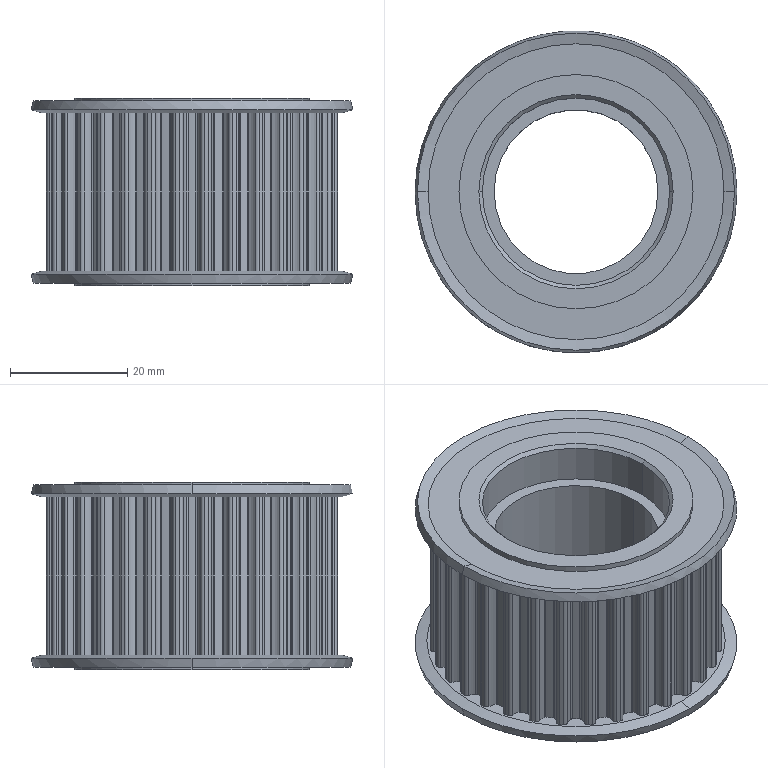Part | SolidWorks | features BaseBody 1 | 1 solid | 319 faces | box 55 x 55 x 32 mm | volume 36284 mm3 | cylinder 295 | cone 16 | plane 8 | commonest cylinder face diameters 1.1 x78 0.5 x74 6.55 x68 46.43 x33 49.97 x32 32 x4